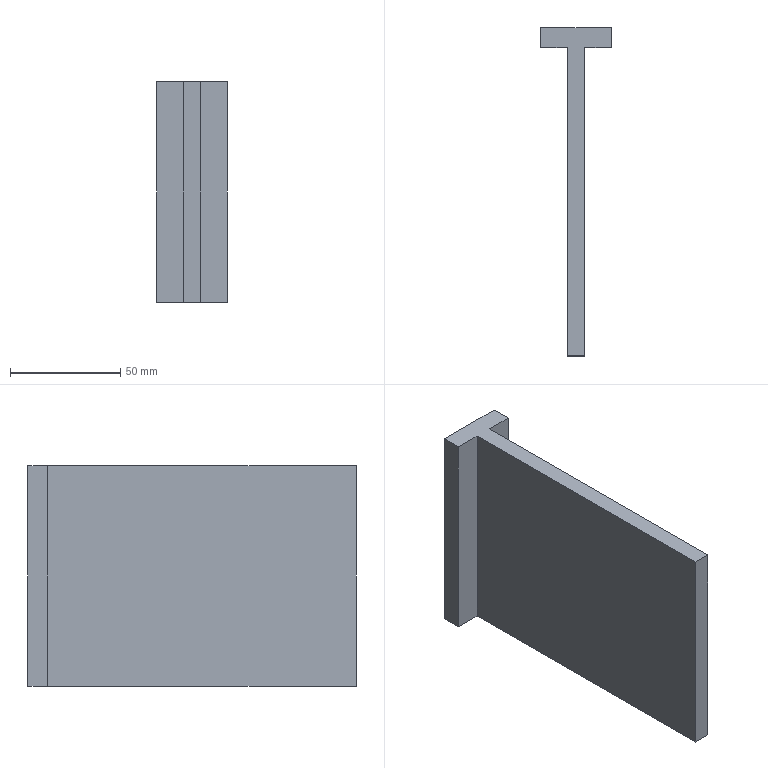Part | SolidWorks | features Extrusion 1 | 1 solid | 10 faces | box 32 x 149 x 100 mm | volume 140800 mm3 | plane 10
STEP:
#1=CARTESIAN_POINT('',(-32.04,-146.512,0.));
#2=VERTEX_POINT('',#1);
#3=CARTESIAN_POINT('',(-24.04,-146.512,0.));
#4=VERTEX_POINT('',#3);
#5=CARTESIAN_POINT('',(-32.04,-146.512,0.));
#6=DIRECTION('',(1.,0.,0.));
#7=VECTOR('',#6,1000.);
#8=LINE('',#5,#7);
#9=EDGE_CURVE('',#2,#4,#8,.T.);
#10=ORIENTED_EDGE('',*,*,#9,.T.);
#11=CARTESIAN_POINT('',(-24.04,-146.512,100.));
#12=VERTEX_POINT('',#11);
#13=CARTESIAN_POINT('',(-24.04,-146.512,100.));
#14=DIRECTION('',(0.,0.,-1.));
#15=VECTOR('',#14,1000.);
#16=LINE('',#13,#15);
#17=EDGE_CURVE('',#12,#4,#16,.T.);
#18=ORIENTED_EDGE('',*,*,#17,.F.);
#19=CARTESIAN_POINT('',(-32.04,-146.512,100.));
#20=VERTEX_POINT('',#19);
#21=CARTESIAN_POINT('',(-32.04,-146.512,100.));
#22=DIRECTION('',(1.,0.,0.));
#23=VECTOR('',#22,1000.);
#24=LINE('',#21,#23);
#25=EDGE_CURVE('',#20,#12,#24,.T.);
#26=ORIENTED_EDGE('',*,*,#25,.F.);
#27=CARTESIAN_POINT('',(-32.04,-146.512,100.));
#28=DIRECTION('',(0.,0.,-1.));
#29=VECTOR('',#28,1000.);
#30=LINE('',#27,#29);
#31=EDGE_CURVE('',#20,#2,#30,.T.);
#32=ORIENTED_EDGE('',*,*,#31,.T.);
#33=EDGE_LOOP('',(#10,#18,#26,#32));
#34=FACE_OUTER_BOUND('',#33,.T.);
#35=CARTESIAN_POINT('',(-32.04,-146.512,100.));
#36=DIRECTION('',(0.,1.,0.));
#37=DIRECTION('',(0.,0.,1.));
#38=AXIS2_PLACEMENT_3D('',#35,#36,#37);
#39=PLANE('',#38);
#40=ADVANCED_FACE('',(#34),#39,.F.);
#41=CARTESIAN_POINT('',(-24.04,-6.512,0.));
#42=VERTEX_POINT('',#41);
#43=CARTESIAN_POINT('',(-24.04,-6.512,0.));
#44=DIRECTION('',(0.,1.,0.));
#45=VECTOR('',#44,1000.);
#46=LINE('',#43,#45);
#47=EDGE_CURVE('',#4,#42,#46,.T.);
#48=ORIENTED_EDGE('',*,*,#47,.T.);
#49=CARTESIAN_POINT('',(-24.04,-6.512,100.));
#50=VERTEX_POINT('',#49);
#51=CARTESIAN_POINT('',(-24.04,-6.512,100.));
#52=DIRECTION('',(0.,0.,-1.));
#53=VECTOR('',#52,1000.);
#54=LINE('',#51,#53);
#55=EDGE_CURVE('',#50,#42,#54,.T.);
#56=ORIENTED_EDGE('',*,*,#55,.F.);
#57=CARTESIAN_POINT('',(-24.04,-120.095,100.));
#58=DIRECTION('',(0.,1.,0.));
#59=VECTOR('',#58,1000.);
#60=LINE('',#57,#59);
#61=EDGE_CURVE('',#12,#50,#60,.T.);
#62=ORIENTED_EDGE('',*,*,#61,.F.);
#63=ORIENTED_EDGE('',*,*,#17,.T.);
#64=EDGE_LOOP('',(#48,#56,#62,#63));
#65=FACE_OUTER_BOUND('',#64,.T.);
#66=CARTESIAN_POINT('',(-24.04,-6.512,100.));
#67=DIRECTION('',(-1.,0.,0.));
#68=DIRECTION('',(0.,-1.,0.));
#69=AXIS2_PLACEMENT_3D('',#66,#67,#68);
#70=PLANE('',#69);
#71=ADVANCED_FACE('',(#65),#70,.F.);
#72=CARTESIAN_POINT('',(-12.04,-6.512,0.));
#73=VERTEX_POINT('',#72);
#74=CARTESIAN_POINT('',(-12.04,-6.512,0.));
#75=DIRECTION('',(1.,0.,0.));
#76=VECTOR('',#75,1000.);
#77=LINE('',#74,#76);
#78=EDGE_CURVE('',#42,#73,#77,.T.);
#79=ORIENTED_EDGE('',*,*,#78,.T.);
#80=CARTESIAN_POINT('',(-12.04,-6.512,100.));
#81=VERTEX_POINT('',#80);
#82=CARTESIAN_POINT('',(-12.04,-6.512,100.));
#83=DIRECTION('',(0.,0.,-1.));
#84=VECTOR('',#83,1000.);
#85=LINE('',#82,#84);
#86=EDGE_CURVE('',#81,#73,#85,.T.);
#87=ORIENTED_EDGE('',*,*,#86,.F.);
#88=CARTESIAN_POINT('',(-12.04,-6.512,100.));
#89=DIRECTION('',(1.,0.,0.));
#90=VECTOR('',#89,1000.);
#91=LINE('',#88,#90);
#92=EDGE_CURVE('',#50,#81,#91,.T.);
#93=ORIENTED_EDGE('',*,*,#92,.F.);
#94=ORIENTED_EDGE('',*,*,#55,.T.);
#95=EDGE_LOOP('',(#79,#87,#93,#94));
#96=FACE_OUTER_BOUND('',#95,.T.);
#97=CARTESIAN_POINT('',(-12.04,-6.512,100.));
#98=DIRECTION('',(0.,1.,0.));
#99=DIRECTION('',(0.,0.,1.));
#100=AXIS2_PLACEMENT_3D('',#97,#98,#99);
#101=PLANE('',#100);
#102=ADVANCED_FACE('',(#96),#101,.F.);
#103=CARTESIAN_POINT('',(-12.04,2.488,0.));
#104=VERTEX_POINT('',#103);
#105=CARTESIAN_POINT('',(-12.04,2.488,0.));
#106=DIRECTION('',(0.,1.,0.));
#107=VECTOR('',#106,1000.);
#108=LINE('',#105,#107);
#109=EDGE_CURVE('',#73,#104,#108,.T.);
#110=ORIENTED_EDGE('',*,*,#109,.T.);
#111=CARTESIAN_POINT('',(-12.04,2.488,100.));
#112=VERTEX_POINT('',#111);
#113=CARTESIAN_POINT('',(-12.04,2.488,100.));
#114=DIRECTION('',(0.,0.,-1.));
#115=VECTOR('',#114,1000.);
#116=LINE('',#113,#115);
#117=EDGE_CURVE('',#112,#104,#116,.T.);
#118=ORIENTED_EDGE('',*,*,#117,.F.);
#119=CARTESIAN_POINT('',(-12.04,2.488,100.));
#120=DIRECTION('',(0.,1.,0.));
#121=VECTOR('',#120,1000.);
#122=LINE('',#119,#121);
#123=EDGE_CURVE('',#81,#112,#122,.T.);
#124=ORIENTED_EDGE('',*,*,#123,.F.);
#125=ORIENTED_EDGE('',*,*,#86,.T.);
#126=EDGE_LOOP('',(#110,#118,#124,#125));
#127=FACE_OUTER_BOUND('',#126,.T.);
#128=CARTESIAN_POINT('',(-12.04,2.488,100.));
#129=DIRECTION('',(-1.,0.,0.));
#130=DIRECTION('',(0.,0.,1.));
#131=AXIS2_PLACEMENT_3D('',#128,#129,#130);
#132=PLANE('',#131);
#133=ADVANCED_FACE('',(#127),#132,.F.);
#134=CARTESIAN_POINT('',(-44.04,2.488,0.));
#135=VERTEX_POINT('',#134);
#136=CARTESIAN_POINT('',(-44.04,2.488,0.));
#137=DIRECTION('',(-1.,0.,0.));
#138=VECTOR('',#137,1000.);
#139=LINE('',#136,#138);
#140=EDGE_CURVE('',#104,#135,#139,.T.);
#141=ORIENTED_EDGE('',*,*,#140,.T.);
#142=CARTESIAN_POINT('',(-44.04,2.488,100.));
#143=VERTEX_POINT('',#142);
#144=CARTESIAN_POINT('',(-44.04,2.488,100.));
#145=DIRECTION('',(0.,0.,-1.));
#146=VECTOR('',#145,1000.);
#147=LINE('',#144,#146);
#148=EDGE_CURVE('',#143,#135,#147,.T.);
#149=ORIENTED_EDGE('',*,*,#148,.F.);
#150=CARTESIAN_POINT('',(-44.04,2.488,100.));
#151=DIRECTION('',(-1.,0.,0.));
#152=VECTOR('',#151,1000.);
#153=LINE('',#150,#152);
#154=EDGE_CURVE('',#112,#143,#153,.T.);
#155=ORIENTED_EDGE('',*,*,#154,.F.);
#156=ORIENTED_EDGE('',*,*,#117,.T.);
#157=EDGE_LOOP('',(#141,#149,#155,#156));
#158=FACE_OUTER_BOUND('',#157,.T.);
#159=CARTESIAN_POINT('',(-44.04,2.488,100.));
#160=DIRECTION('',(0.,-1.,0.));
#161=DIRECTION('',(0.,0.,-1.));
#162=AXIS2_PLACEMENT_3D('',#159,#160,#161);
#163=PLANE('',#162);
#164=ADVANCED_FACE('',(#158),#163,.F.);
#165=CARTESIAN_POINT('',(-44.04,-6.512,0.));
#166=VERTEX_POINT('',#165);
#167=CARTESIAN_POINT('',(-44.04,2.488,0.));
#168=DIRECTION('',(0.,-1.,0.));
#169=VECTOR('',#168,1000.);
#170=LINE('',#167,#169);
#171=EDGE_CURVE('',#135,#166,#170,.T.);
#172=ORIENTED_EDGE('',*,*,#171,.T.);
#173=CARTESIAN_POINT('',(-44.04,-6.512,100.));
#174=VERTEX_POINT('',#173);
#175=CARTESIAN_POINT('',(-44.04,-6.512,100.));
#176=DIRECTION('',(0.,0.,-1.));
#177=VECTOR('',#176,1000.);
#178=LINE('',#175,#177);
#179=EDGE_CURVE('',#174,#166,#178,.T.);
#180=ORIENTED_EDGE('',*,*,#179,.F.);
#181=CARTESIAN_POINT('',(-44.04,2.488,100.));
#182=DIRECTION('',(0.,-1.,0.));
#183=VECTOR('',#182,1000.);
#184=LINE('',#181,#183);
#185=EDGE_CURVE('',#143,#174,#184,.T.);
#186=ORIENTED_EDGE('',*,*,#185,.F.);
#187=ORIENTED_EDGE('',*,*,#148,.T.);
#188=EDGE_LOOP('',(#172,#180,#186,#187));
#189=FACE_OUTER_BOUND('',#188,.T.);
#190=CARTESIAN_POINT('',(-44.04,2.488,100.));
#191=DIRECTION('',(1.,0.,0.));
#192=DIRECTION('',(0.,0.,-1.));
#193=AXIS2_PLACEMENT_3D('',#190,#191,#192);
#194=PLANE('',#193);
#195=ADVANCED_FACE('',(#189),#194,.F.);
#196=CARTESIAN_POINT('',(-32.04,-6.512,0.));
#197=VERTEX_POINT('',#196);
#198=CARTESIAN_POINT('',(-44.04,-6.512,0.));
#199=DIRECTION('',(1.,0.,0.));
#200=VECTOR('',#199,1000.);
#201=LINE('',#198,#200);
#202=EDGE_CURVE('',#166,#197,#201,.T.);
#203=ORIENTED_EDGE('',*,*,#202,.T.);
#204=CARTESIAN_POINT('',(-32.04,-6.512,100.));
#205=VERTEX_POINT('',#204);
#206=CARTESIAN_POINT('',(-32.04,-6.512,100.));
#207=DIRECTION('',(0.,0.,-1.));
#208=VECTOR('',#207,1000.);
#209=LINE('',#206,#208);
#210=EDGE_CURVE('',#205,#197,#209,.T.);
#211=ORIENTED_EDGE('',*,*,#210,.F.);
#212=CARTESIAN_POINT('',(-44.04,-6.512,100.));
#213=DIRECTION('',(1.,0.,0.));
#214=VECTOR('',#213,1000.);
#215=LINE('',#212,#214);
#216=EDGE_CURVE('',#174,#205,#215,.T.);
#217=ORIENTED_EDGE('',*,*,#216,.F.);
#218=ORIENTED_EDGE('',*,*,#179,.T.);
#219=EDGE_LOOP('',(#203,#211,#217,#218));
#220=FACE_OUTER_BOUND('',#219,.T.);
#221=CARTESIAN_POINT('',(-44.04,-6.512,100.));
#222=DIRECTION('',(0.,1.,0.));
#223=DIRECTION('',(0.,0.,1.));
#224=AXIS2_PLACEMENT_3D('',#221,#222,#223);
#225=PLANE('',#224);
#226=ADVANCED_FACE('',(#220),#225,.F.);
#227=CARTESIAN_POINT('',(-32.04,-120.095,0.));
#228=DIRECTION('',(0.,-1.,0.));
#229=VECTOR('',#228,1000.);
#230=LINE('',#227,#229);
#231=EDGE_CURVE('',#197,#2,#230,.T.);
#232=ORIENTED_EDGE('',*,*,#231,.T.);
#233=ORIENTED_EDGE('',*,*,#31,.F.);
#234=CARTESIAN_POINT('',(-32.04,-6.512,100.));
#235=DIRECTION('',(0.,-1.,0.));
#236=VECTOR('',#235,1000.);
#237=LINE('',#234,#236);
#238=EDGE_CURVE('',#205,#20,#237,.T.);
#239=ORIENTED_EDGE('',*,*,#238,.F.);
#240=ORIENTED_EDGE('',*,*,#210,.T.);
#241=EDGE_LOOP('',(#232,#233,#239,#240));
#242=FACE_OUTER_BOUND('',#241,.T.);
#243=CARTESIAN_POINT('',(-32.04,-120.095,100.));
#244=DIRECTION('',(1.,0.,0.));
#245=DIRECTION('',(0.,0.,-1.));
#246=AXIS2_PLACEMENT_3D('',#243,#244,#245);
#247=PLANE('',#246);
#248=ADVANCED_FACE('',(#242),#247,.F.);
#249=ORIENTED_EDGE('',*,*,#25,.T.);
#250=ORIENTED_EDGE('',*,*,#61,.T.);
#251=ORIENTED_EDGE('',*,*,#92,.T.);
#252=ORIENTED_EDGE('',*,*,#123,.T.);
#253=ORIENTED_EDGE('',*,*,#154,.T.);
#254=ORIENTED_EDGE('',*,*,#185,.T.);
#255=ORIENTED_EDGE('',*,*,#216,.T.);
#256=ORIENTED_EDGE('',*,*,#238,.T.);
#257=EDGE_LOOP('',(#249,#250,#251,#252,#253,#254,#255,#256));
#258=FACE_OUTER_BOUND('',#257,.T.);
#259=CARTESIAN_POINT('',(0.,0.,100.));
#260=DIRECTION('',(0.,0.,-1.));
#261=DIRECTION('',(-1.,0.,0.));
#262=AXIS2_PLACEMENT_3D('',#259,#260,#261);
#263=PLANE('',#262);
#264=ADVANCED_FACE('',(#258),#263,.F.);
#265=ORIENTED_EDGE('',*,*,#9,.F.);
#266=ORIENTED_EDGE('',*,*,#231,.F.);
#267=ORIENTED_EDGE('',*,*,#202,.F.);
#268=ORIENTED_EDGE('',*,*,#171,.F.);
#269=ORIENTED_EDGE('',*,*,#140,.F.);
#270=ORIENTED_EDGE('',*,*,#109,.F.);
#271=ORIENTED_EDGE('',*,*,#78,.F.);
#272=ORIENTED_EDGE('',*,*,#47,.F.);
#273=EDGE_LOOP('',(#265,#266,#267,#268,#269,#270,#271,#272));
#274=FACE_OUTER_BOUND('',#273,.T.);
#275=CARTESIAN_POINT('',(0.,0.,0.));
#276=DIRECTION('',(0.,0.,-1.));
#277=DIRECTION('',(-1.,0.,0.));
#278=AXIS2_PLACEMENT_3D('',#275,#276,#277);
#279=PLANE('',#278);
#280=ADVANCED_FACE('',(#274),#279,.T.);
#281=CLOSED_SHELL('',(#40,#71,#102,#133,#164,#195,#226,#248,#264,#280));
#282=MANIFOLD_SOLID_BREP('',#281);
#283=CARTESIAN_POINT('',(0.,0.,0.));
#284=DIRECTION('',(0.,0.,1.));
#285=DIRECTION('',(1.,0.,0.));
#286=AXIS2_PLACEMENT_3D('',#283,#284,#285);
#287=(LENGTH_UNIT()NAMED_UNIT(*)SI_UNIT(.MILLI.,.METRE.));
#288=UNCERTAINTY_MEASURE_WITH_UNIT(LENGTH_MEASURE(0.00001),#287,'','');
#289=(NAMED_UNIT(*)PLANE_ANGLE_UNIT()SI_UNIT($,.RADIAN.));
#290=(NAMED_UNIT(*)SI_UNIT($,.STERADIAN.)SOLID_ANGLE_UNIT());
#291=(GEOMETRIC_REPRESENTATION_CONTEXT(3)GLOBAL_UNCERTAINTY_ASSIGNED_CONTEXT((#288))GLOBAL_UNIT_ASSIGNED_CONTEXT((#287,#289,#290))REPRESENTATION_CONTEXT('',''));
#292=ADVANCED_BREP_SHAPE_REPRESENTATION('',(#282,#286),#291);